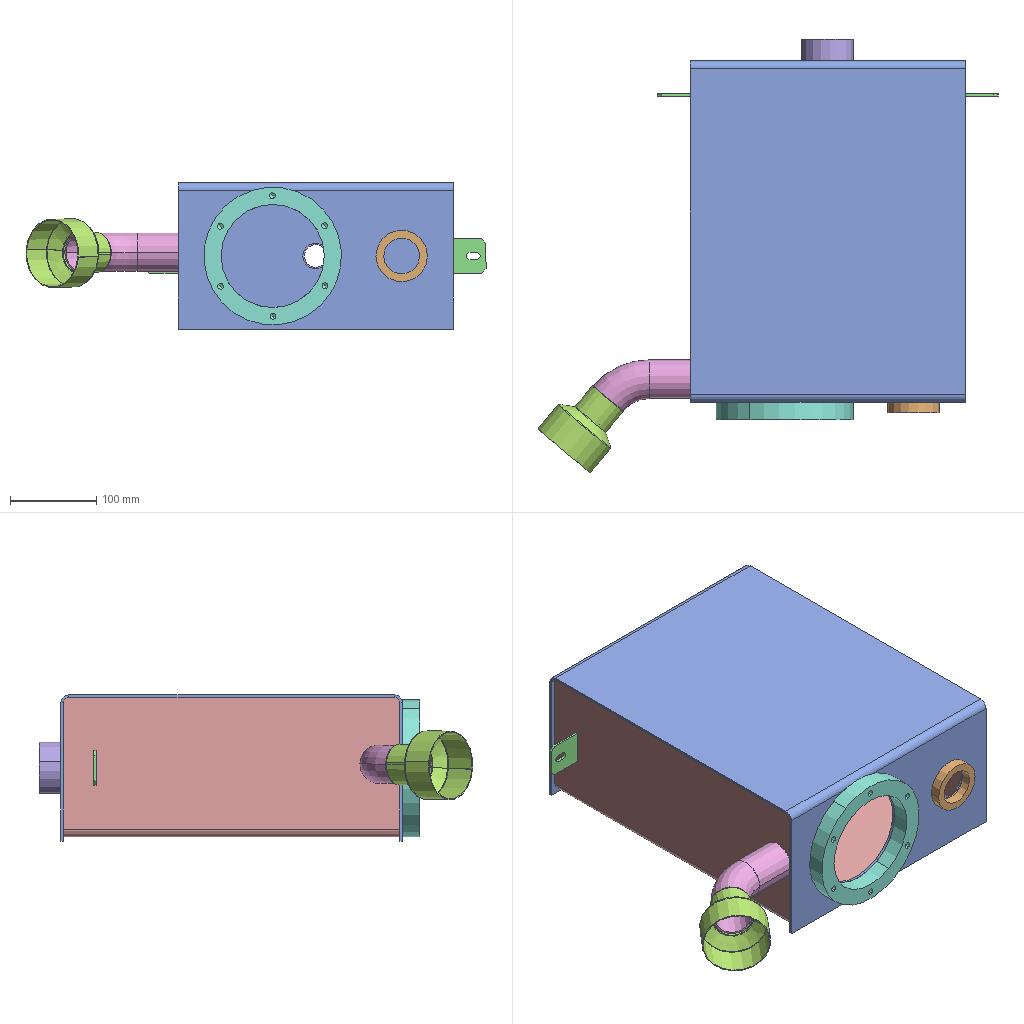Assembly | SolidWorks | 8 different items | 9 placed | box 535 x 504 x 170 mm
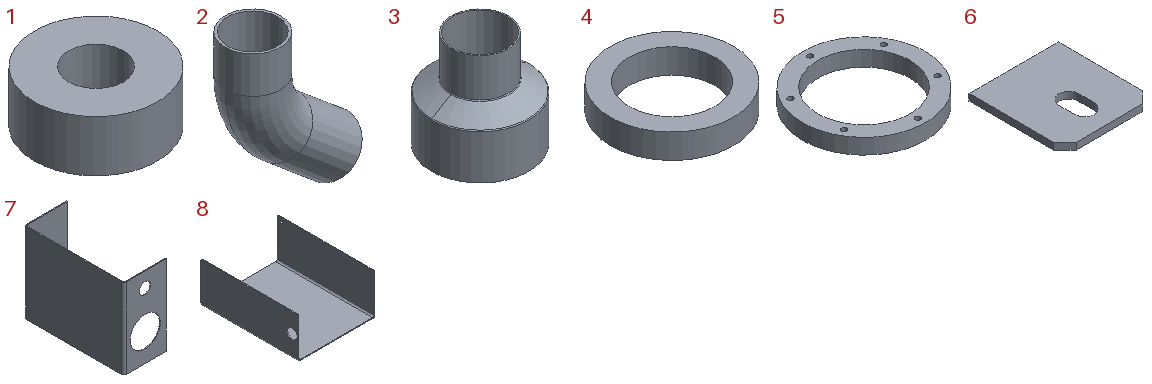Parts list (item | quantity | size | volume | features):
1 | x1 | 60 x 60 x 25 mm | 56897 mm3 | features 3DProfileFeature 1, Extrusion 1, HoleWzd 1
2 | x1 | 99.465 x 45 x 128.591 mm | 36956 mm3 | features Shell 1, Sweep 1
3 | x1 | 80 x 80 x 79 mm | 17561 mm3 | features 3DProfileFeature 2, ICE 2, Blend 1, Fillet 1, Shell 1
4 | x1 | 60 x 60 x 12 mm | 17462 mm3 | features Extrusion 1
5 | x1 | 160 x 160 x 20 mm | 171859 mm3 | features 3DProfileFeature 1, Extrusion 1, HoleWzd 1
6 | x2 | 40 x 43 x 3 mm | 4705 mm3 | features Extrusion 1
7 | x1 | 170 x 397 x 320 mm | 654758 mm3 | features Cut 2, FlatPattern 1, SMBaseFlange 1, SheetMetal 1
8 | x1 | 310 x 391 x 162 mm | 724944 mm3 | features Cut 2, FlatPattern 1, ICE 1, SMBaseFlange 1, SheetMetal 1
Mates (type | each side: item.copy, entity, surface, feature):
Coincident | 8.1 face plane Base-Flange1 | 7.1 face plane Base-Flange1 | 2 times
DistanceDim | 8.1 face plane Base-Flange1 | 7.1 face plane Base-Flange1
Concentric | 8.1 edge | 2.1 edge
Coincident | 8.1 face plane Base-Flange1 | 2.1 face plane Sweep1
Concentric | 3.1 edge | 2.1 edge
Coincident | 7.1 edge | 5.1 edge
Concentric | 7.1 edge | 4.1 edge
Coincident | 7.1 face plane Base-Flange1 | 4.1 face plane Boss-Extrude1
Concentric | 7.1 edge | 1.1 edge
Coincident | 7.1 face plane Base-Flange1 | 1.1 face plane Boss-Extrude1
DistanceDim | 6.1 face plane Boss-Extrude1 | 7.1 face plane Base-Flange1
Coincident | 8.1 face plane Base-Flange1 | 6.1 face plane Boss-Extrude1
Coincident | 6.1 face plane Boss-Extrude1 | assembly select_type:10
Coincident | 6.1 face plane Boss-Extrude1 | 6.2 face plane Boss-Extrude1 | 2 times
Coincident | 8.1 face plane Base-Flange1 | 6.2 face plane Boss-Extrude1